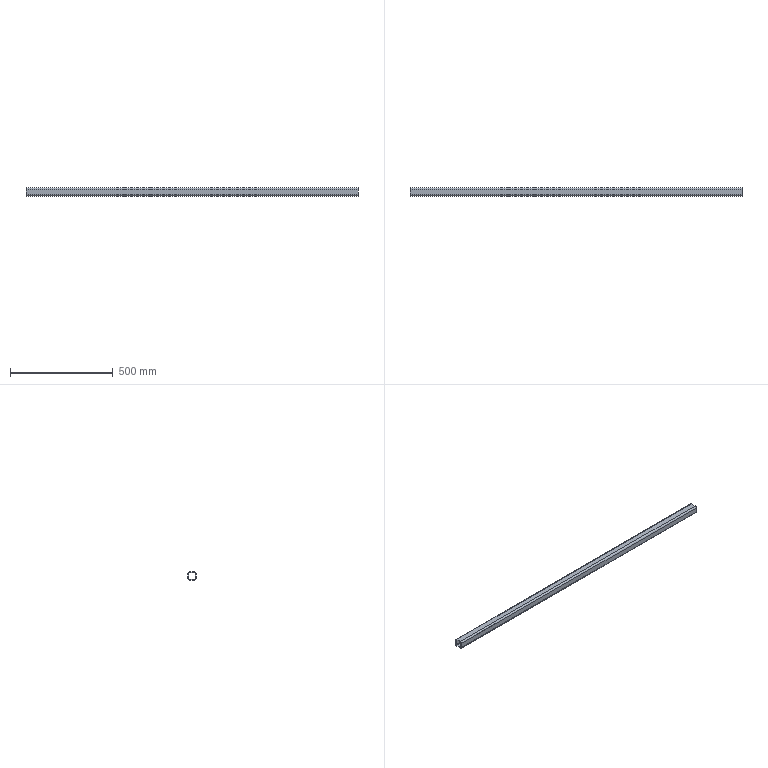Part | STEP file | Microwave Drying Flat Conveyor-CN2500x400-105-102_Default<Machining blank> | 1 solid | 18 faces | box 1612 x 40 x 40 mm | volume 862092 mm3 | plane 10 | cylinder 8 | commonest cylinder face diameters 8 x4 16 x4
STEP:
#1=CARTESIAN_POINT('',(0.,-20.,12.));
#2=VERTEX_POINT('',#1);
#3=CARTESIAN_POINT('',(0.,-12.,20.));
#4=VERTEX_POINT('',#3);
#5=CARTESIAN_POINT('',(0.,-12.,12.));
#6=DIRECTION('',(-1.,0.,0.));
#7=DIRECTION('',(0.,-1.,0.));
#8=AXIS2_PLACEMENT_3D('',#5,#6,#7);
#9=CIRCLE('',#8,8.);
#10=EDGE_CURVE('',#2,#4,#9,.T.);
#11=ORIENTED_EDGE('',*,*,#10,.T.);
#12=CARTESIAN_POINT('',(-1612.,-12.,20.));
#13=VERTEX_POINT('',#12);
#14=CARTESIAN_POINT('',(-1612.,-12.,20.));
#15=DIRECTION('',(1.,0.,0.));
#16=VECTOR('',#15,1000.);
#17=LINE('',#14,#16);
#18=EDGE_CURVE('',#13,#4,#17,.T.);
#19=ORIENTED_EDGE('',*,*,#18,.F.);
#20=CARTESIAN_POINT('',(-1612.,-20.,12.));
#21=VERTEX_POINT('',#20);
#22=CARTESIAN_POINT('',(-1612.,-12.,12.));
#23=DIRECTION('',(-1.,0.,0.));
#24=DIRECTION('',(0.,-1.,0.));
#25=AXIS2_PLACEMENT_3D('',#22,#23,#24);
#26=CIRCLE('',#25,8.);
#27=EDGE_CURVE('',#21,#13,#26,.T.);
#28=ORIENTED_EDGE('',*,*,#27,.F.);
#29=CARTESIAN_POINT('',(-1612.,-20.,12.));
#30=DIRECTION('',(1.,0.,0.));
#31=VECTOR('',#30,1000.);
#32=LINE('',#29,#31);
#33=EDGE_CURVE('',#21,#2,#32,.T.);
#34=ORIENTED_EDGE('',*,*,#33,.T.);
#35=EDGE_LOOP('',(#11,#19,#28,#34));
#36=FACE_OUTER_BOUND('',#35,.T.);
#37=CARTESIAN_POINT('',(-1612.,-12.,12.));
#38=DIRECTION('',(1.,0.,0.));
#39=DIRECTION('',(0.,1.,0.));
#40=AXIS2_PLACEMENT_3D('',#37,#38,#39);
#41=CYLINDRICAL_SURFACE('',#40,8.);
#42=ADVANCED_FACE('',(#36),#41,.T.);
#43=CARTESIAN_POINT('',(0.,12.,20.));
#44=VERTEX_POINT('',#43);
#45=CARTESIAN_POINT('',(0.,-12.,20.));
#46=DIRECTION('',(0.,1.,0.));
#47=VECTOR('',#46,1000.);
#48=LINE('',#45,#47);
#49=EDGE_CURVE('',#4,#44,#48,.T.);
#50=ORIENTED_EDGE('',*,*,#49,.T.);
#51=CARTESIAN_POINT('',(-1612.,12.,20.));
#52=VERTEX_POINT('',#51);
#53=CARTESIAN_POINT('',(-1612.,12.,20.));
#54=DIRECTION('',(1.,0.,0.));
#55=VECTOR('',#54,1000.);
#56=LINE('',#53,#55);
#57=EDGE_CURVE('',#52,#44,#56,.T.);
#58=ORIENTED_EDGE('',*,*,#57,.F.);
#59=CARTESIAN_POINT('',(-1612.,-12.,20.));
#60=DIRECTION('',(0.,1.,0.));
#61=VECTOR('',#60,1000.);
#62=LINE('',#59,#61);
#63=EDGE_CURVE('',#13,#52,#62,.T.);
#64=ORIENTED_EDGE('',*,*,#63,.F.);
#65=ORIENTED_EDGE('',*,*,#18,.T.);
#66=EDGE_LOOP('',(#50,#58,#64,#65));
#67=FACE_OUTER_BOUND('',#66,.T.);
#68=CARTESIAN_POINT('',(-1612.,-12.,20.));
#69=DIRECTION('',(0.,0.,-1.));
#70=DIRECTION('',(-1.,0.,0.));
#71=AXIS2_PLACEMENT_3D('',#68,#69,#70);
#72=PLANE('',#71);
#73=ADVANCED_FACE('',(#67),#72,.F.);
#74=CARTESIAN_POINT('',(0.,20.,12.));
#75=VERTEX_POINT('',#74);
#76=CARTESIAN_POINT('',(0.,12.,12.));
#77=DIRECTION('',(-1.,0.,0.));
#78=DIRECTION('',(0.,-1.,0.));
#79=AXIS2_PLACEMENT_3D('',#76,#77,#78);
#80=CIRCLE('',#79,8.);
#81=EDGE_CURVE('',#44,#75,#80,.T.);
#82=ORIENTED_EDGE('',*,*,#81,.T.);
#83=CARTESIAN_POINT('',(-1612.,20.,12.));
#84=VERTEX_POINT('',#83);
#85=CARTESIAN_POINT('',(-1612.,20.,12.));
#86=DIRECTION('',(1.,0.,0.));
#87=VECTOR('',#86,1000.);
#88=LINE('',#85,#87);
#89=EDGE_CURVE('',#84,#75,#88,.T.);
#90=ORIENTED_EDGE('',*,*,#89,.F.);
#91=CARTESIAN_POINT('',(-1612.,12.,12.));
#92=DIRECTION('',(-1.,0.,0.));
#93=DIRECTION('',(0.,-1.,0.));
#94=AXIS2_PLACEMENT_3D('',#91,#92,#93);
#95=CIRCLE('',#94,8.);
#96=EDGE_CURVE('',#52,#84,#95,.T.);
#97=ORIENTED_EDGE('',*,*,#96,.F.);
#98=ORIENTED_EDGE('',*,*,#57,.T.);
#99=EDGE_LOOP('',(#82,#90,#97,#98));
#100=FACE_OUTER_BOUND('',#99,.T.);
#101=CARTESIAN_POINT('',(-1612.,12.,12.));
#102=DIRECTION('',(1.,0.,0.));
#103=DIRECTION('',(0.,1.,0.));
#104=AXIS2_PLACEMENT_3D('',#101,#102,#103);
#105=CYLINDRICAL_SURFACE('',#104,8.);
#106=ADVANCED_FACE('',(#100),#105,.T.);
#107=CARTESIAN_POINT('',(0.,20.,-12.));
#108=VERTEX_POINT('',#107);
#109=CARTESIAN_POINT('',(0.,20.,-12.));
#110=DIRECTION('',(0.,0.,-1.));
#111=VECTOR('',#110,1000.);
#112=LINE('',#109,#111);
#113=EDGE_CURVE('',#75,#108,#112,.T.);
#114=ORIENTED_EDGE('',*,*,#113,.T.);
#115=CARTESIAN_POINT('',(-1612.,20.,-12.));
#116=VERTEX_POINT('',#115);
#117=CARTESIAN_POINT('',(-1612.,20.,-12.));
#118=DIRECTION('',(1.,0.,0.));
#119=VECTOR('',#118,1000.);
#120=LINE('',#117,#119);
#121=EDGE_CURVE('',#116,#108,#120,.T.);
#122=ORIENTED_EDGE('',*,*,#121,.F.);
#123=CARTESIAN_POINT('',(-1612.,20.,-12.));
#124=DIRECTION('',(0.,0.,-1.));
#125=VECTOR('',#124,1000.);
#126=LINE('',#123,#125);
#127=EDGE_CURVE('',#84,#116,#126,.T.);
#128=ORIENTED_EDGE('',*,*,#127,.F.);
#129=ORIENTED_EDGE('',*,*,#89,.T.);
#130=EDGE_LOOP('',(#114,#122,#128,#129));
#131=FACE_OUTER_BOUND('',#130,.T.);
#132=CARTESIAN_POINT('',(-1612.,20.,-12.));
#133=DIRECTION('',(0.,-1.,0.));
#134=DIRECTION('',(1.,0.,0.));
#135=AXIS2_PLACEMENT_3D('',#132,#133,#134);
#136=PLANE('',#135);
#137=ADVANCED_FACE('',(#131),#136,.F.);
#138=CARTESIAN_POINT('',(0.,12.,-20.));
#139=VERTEX_POINT('',#138);
#140=CARTESIAN_POINT('',(0.,12.,-12.));
#141=DIRECTION('',(-1.,0.,0.));
#142=DIRECTION('',(0.,-1.,0.));
#143=AXIS2_PLACEMENT_3D('',#140,#141,#142);
#144=CIRCLE('',#143,8.);
#145=EDGE_CURVE('',#108,#139,#144,.T.);
#146=ORIENTED_EDGE('',*,*,#145,.T.);
#147=CARTESIAN_POINT('',(-1612.,12.,-20.));
#148=VERTEX_POINT('',#147);
#149=CARTESIAN_POINT('',(-1612.,12.,-20.));
#150=DIRECTION('',(1.,0.,0.));
#151=VECTOR('',#150,1000.);
#152=LINE('',#149,#151);
#153=EDGE_CURVE('',#148,#139,#152,.T.);
#154=ORIENTED_EDGE('',*,*,#153,.F.);
#155=CARTESIAN_POINT('',(-1612.,12.,-12.));
#156=DIRECTION('',(-1.,0.,0.));
#157=DIRECTION('',(0.,-1.,0.));
#158=AXIS2_PLACEMENT_3D('',#155,#156,#157);
#159=CIRCLE('',#158,8.);
#160=EDGE_CURVE('',#116,#148,#159,.T.);
#161=ORIENTED_EDGE('',*,*,#160,.F.);
#162=ORIENTED_EDGE('',*,*,#121,.T.);
#163=EDGE_LOOP('',(#146,#154,#161,#162));
#164=FACE_OUTER_BOUND('',#163,.T.);
#165=CARTESIAN_POINT('',(-1612.,12.,-12.));
#166=DIRECTION('',(1.,0.,0.));
#167=DIRECTION('',(0.,1.,0.));
#168=AXIS2_PLACEMENT_3D('',#165,#166,#167);
#169=CYLINDRICAL_SURFACE('',#168,8.);
#170=ADVANCED_FACE('',(#164),#169,.T.);
#171=CARTESIAN_POINT('',(0.,-12.,-20.));
#172=VERTEX_POINT('',#171);
#173=CARTESIAN_POINT('',(0.,12.,-20.));
#174=DIRECTION('',(0.,-1.,0.));
#175=VECTOR('',#174,1000.);
#176=LINE('',#173,#175);
#177=EDGE_CURVE('',#139,#172,#176,.T.);
#178=ORIENTED_EDGE('',*,*,#177,.T.);
#179=CARTESIAN_POINT('',(-1612.,-12.,-20.));
#180=VERTEX_POINT('',#179);
#181=CARTESIAN_POINT('',(-1612.,-12.,-20.));
#182=DIRECTION('',(1.,0.,0.));
#183=VECTOR('',#182,1000.);
#184=LINE('',#181,#183);
#185=EDGE_CURVE('',#180,#172,#184,.T.);
#186=ORIENTED_EDGE('',*,*,#185,.F.);
#187=CARTESIAN_POINT('',(-1612.,12.,-20.));
#188=DIRECTION('',(0.,-1.,0.));
#189=VECTOR('',#188,1000.);
#190=LINE('',#187,#189);
#191=EDGE_CURVE('',#148,#180,#190,.T.);
#192=ORIENTED_EDGE('',*,*,#191,.F.);
#193=ORIENTED_EDGE('',*,*,#153,.T.);
#194=EDGE_LOOP('',(#178,#186,#192,#193));
#195=FACE_OUTER_BOUND('',#194,.T.);
#196=CARTESIAN_POINT('',(-1612.,12.,-20.));
#197=DIRECTION('',(0.,0.,1.));
#198=DIRECTION('',(1.,0.,0.));
#199=AXIS2_PLACEMENT_3D('',#196,#197,#198);
#200=PLANE('',#199);
#201=ADVANCED_FACE('',(#195),#200,.F.);
#202=CARTESIAN_POINT('',(0.,-20.,-12.));
#203=VERTEX_POINT('',#202);
#204=CARTESIAN_POINT('',(0.,-12.,-12.));
#205=DIRECTION('',(-1.,0.,0.));
#206=DIRECTION('',(0.,-1.,0.));
#207=AXIS2_PLACEMENT_3D('',#204,#205,#206);
#208=CIRCLE('',#207,8.);
#209=EDGE_CURVE('',#172,#203,#208,.T.);
#210=ORIENTED_EDGE('',*,*,#209,.T.);
#211=CARTESIAN_POINT('',(-1612.,-20.,-12.));
#212=VERTEX_POINT('',#211);
#213=CARTESIAN_POINT('',(-1612.,-20.,-12.));
#214=DIRECTION('',(1.,0.,0.));
#215=VECTOR('',#214,1000.);
#216=LINE('',#213,#215);
#217=EDGE_CURVE('',#212,#203,#216,.T.);
#218=ORIENTED_EDGE('',*,*,#217,.F.);
#219=CARTESIAN_POINT('',(-1612.,-12.,-12.));
#220=DIRECTION('',(-1.,0.,0.));
#221=DIRECTION('',(0.,-1.,0.));
#222=AXIS2_PLACEMENT_3D('',#219,#220,#221);
#223=CIRCLE('',#222,8.);
#224=EDGE_CURVE('',#180,#212,#223,.T.);
#225=ORIENTED_EDGE('',*,*,#224,.F.);
#226=ORIENTED_EDGE('',*,*,#185,.T.);
#227=EDGE_LOOP('',(#210,#218,#225,#226));
#228=FACE_OUTER_BOUND('',#227,.T.);
#229=CARTESIAN_POINT('',(-1612.,-12.,-12.));
#230=DIRECTION('',(1.,0.,0.));
#231=DIRECTION('',(0.,1.,0.));
#232=AXIS2_PLACEMENT_3D('',#229,#230,#231);
#233=CYLINDRICAL_SURFACE('',#232,8.);
#234=ADVANCED_FACE('',(#228),#233,.T.);
#235=CARTESIAN_POINT('',(0.,12.,16.));
#236=VERTEX_POINT('',#235);
#237=CARTESIAN_POINT('',(0.,16.,12.));
#238=VERTEX_POINT('',#237);
#239=CARTESIAN_POINT('',(0.,12.,12.));
#240=DIRECTION('',(-1.,0.,0.));
#241=DIRECTION('',(0.,-1.,0.));
#242=AXIS2_PLACEMENT_3D('',#239,#240,#241);
#243=CIRCLE('',#242,4.);
#244=EDGE_CURVE('',#236,#238,#243,.T.);
#245=ORIENTED_EDGE('',*,*,#244,.F.);
#246=CARTESIAN_POINT('',(-1612.,12.,16.));
#247=VERTEX_POINT('',#246);
#248=CARTESIAN_POINT('',(-1612.,12.,16.));
#249=DIRECTION('',(1.,0.,0.));
#250=VECTOR('',#249,1000.);
#251=LINE('',#248,#250);
#252=EDGE_CURVE('',#247,#236,#251,.T.);
#253=ORIENTED_EDGE('',*,*,#252,.F.);
#254=CARTESIAN_POINT('',(-1612.,16.,12.));
#255=VERTEX_POINT('',#254);
#256=CARTESIAN_POINT('',(-1612.,12.,12.));
#257=DIRECTION('',(-1.,0.,0.));
#258=DIRECTION('',(0.,-1.,0.));
#259=AXIS2_PLACEMENT_3D('',#256,#257,#258);
#260=CIRCLE('',#259,4.);
#261=EDGE_CURVE('',#247,#255,#260,.T.);
#262=ORIENTED_EDGE('',*,*,#261,.T.);
#263=CARTESIAN_POINT('',(-1612.,16.,12.));
#264=DIRECTION('',(1.,0.,0.));
#265=VECTOR('',#264,1000.);
#266=LINE('',#263,#265);
#267=EDGE_CURVE('',#255,#238,#266,.T.);
#268=ORIENTED_EDGE('',*,*,#267,.T.);
#269=EDGE_LOOP('',(#245,#253,#262,#268));
#270=FACE_OUTER_BOUND('',#269,.T.);
#271=CARTESIAN_POINT('',(-1612.,12.,12.));
#272=DIRECTION('',(1.,0.,0.));
#273=DIRECTION('',(0.,1.,0.));
#274=AXIS2_PLACEMENT_3D('',#271,#272,#273);
#275=CYLINDRICAL_SURFACE('',#274,4.);
#276=ADVANCED_FACE('',(#270),#275,.F.);
#277=CARTESIAN_POINT('',(0.,-12.,16.));
#278=VERTEX_POINT('',#277);
#279=CARTESIAN_POINT('',(0.,-12.,16.));
#280=DIRECTION('',(0.,1.,0.));
#281=VECTOR('',#280,1000.);
#282=LINE('',#279,#281);
#283=EDGE_CURVE('',#278,#236,#282,.T.);
#284=ORIENTED_EDGE('',*,*,#283,.F.);
#285=CARTESIAN_POINT('',(-1612.,-12.,16.));
#286=VERTEX_POINT('',#285);
#287=CARTESIAN_POINT('',(-1612.,-12.,16.));
#288=DIRECTION('',(1.,0.,0.));
#289=VECTOR('',#288,1000.);
#290=LINE('',#287,#289);
#291=EDGE_CURVE('',#286,#278,#290,.T.);
#292=ORIENTED_EDGE('',*,*,#291,.F.);
#293=CARTESIAN_POINT('',(-1612.,-12.,16.));
#294=DIRECTION('',(0.,1.,0.));
#295=VECTOR('',#294,1000.);
#296=LINE('',#293,#295);
#297=EDGE_CURVE('',#286,#247,#296,.T.);
#298=ORIENTED_EDGE('',*,*,#297,.T.);
#299=ORIENTED_EDGE('',*,*,#252,.T.);
#300=EDGE_LOOP('',(#284,#292,#298,#299));
#301=FACE_OUTER_BOUND('',#300,.T.);
#302=CARTESIAN_POINT('',(-1612.,-12.,16.));
#303=DIRECTION('',(0.,0.,-1.));
#304=DIRECTION('',(-1.,0.,0.));
#305=AXIS2_PLACEMENT_3D('',#302,#303,#304);
#306=PLANE('',#305);
#307=ADVANCED_FACE('',(#301),#306,.T.);
#308=CARTESIAN_POINT('',(0.,-16.,12.));
#309=VERTEX_POINT('',#308);
#310=CARTESIAN_POINT('',(0.,-12.,12.));
#311=DIRECTION('',(-1.,0.,0.));
#312=DIRECTION('',(0.,-1.,0.));
#313=AXIS2_PLACEMENT_3D('',#310,#311,#312);
#314=CIRCLE('',#313,4.);
#315=EDGE_CURVE('',#309,#278,#314,.T.);
#316=ORIENTED_EDGE('',*,*,#315,.F.);
#317=CARTESIAN_POINT('',(-1612.,-16.,12.));
#318=VERTEX_POINT('',#317);
#319=CARTESIAN_POINT('',(-1612.,-16.,12.));
#320=DIRECTION('',(1.,0.,0.));
#321=VECTOR('',#320,1000.);
#322=LINE('',#319,#321);
#323=EDGE_CURVE('',#318,#309,#322,.T.);
#324=ORIENTED_EDGE('',*,*,#323,.F.);
#325=CARTESIAN_POINT('',(-1612.,-12.,12.));
#326=DIRECTION('',(-1.,0.,0.));
#327=DIRECTION('',(0.,-1.,0.));
#328=AXIS2_PLACEMENT_3D('',#325,#326,#327);
#329=CIRCLE('',#328,4.);
#330=EDGE_CURVE('',#318,#286,#329,.T.);
#331=ORIENTED_EDGE('',*,*,#330,.T.);
#332=ORIENTED_EDGE('',*,*,#291,.T.);
#333=EDGE_LOOP('',(#316,#324,#331,#332));
#334=FACE_OUTER_BOUND('',#333,.T.);
#335=CARTESIAN_POINT('',(-1612.,-12.,12.));
#336=DIRECTION('',(1.,0.,0.));
#337=DIRECTION('',(0.,1.,0.));
#338=AXIS2_PLACEMENT_3D('',#335,#336,#337);
#339=CYLINDRICAL_SURFACE('',#338,4.);
#340=ADVANCED_FACE('',(#334),#339,.F.);
#341=CARTESIAN_POINT('',(0.,-16.,-12.));
#342=VERTEX_POINT('',#341);
#343=CARTESIAN_POINT('',(0.,-16.,12.));
#344=DIRECTION('',(0.,0.,1.));
#345=VECTOR('',#344,1000.);
#346=LINE('',#343,#345);
#347=EDGE_CURVE('',#342,#309,#346,.T.);
#348=ORIENTED_EDGE('',*,*,#347,.F.);
#349=CARTESIAN_POINT('',(-1612.,-16.,-12.));
#350=VERTEX_POINT('',#349);
#351=CARTESIAN_POINT('',(-1612.,-16.,-12.));
#352=DIRECTION('',(1.,0.,0.));
#353=VECTOR('',#352,1000.);
#354=LINE('',#351,#353);
#355=EDGE_CURVE('',#350,#342,#354,.T.);
#356=ORIENTED_EDGE('',*,*,#355,.F.);
#357=CARTESIAN_POINT('',(-1612.,-16.,12.));
#358=DIRECTION('',(0.,0.,1.));
#359=VECTOR('',#358,1000.);
#360=LINE('',#357,#359);
#361=EDGE_CURVE('',#350,#318,#360,.T.);
#362=ORIENTED_EDGE('',*,*,#361,.T.);
#363=ORIENTED_EDGE('',*,*,#323,.T.);
#364=EDGE_LOOP('',(#348,#356,#362,#363));
#365=FACE_OUTER_BOUND('',#364,.T.);
#366=CARTESIAN_POINT('',(-1612.,-16.,12.));
#367=DIRECTION('',(0.,1.,0.));
#368=DIRECTION('',(-1.,0.,0.));
#369=AXIS2_PLACEMENT_3D('',#366,#367,#368);
#370=PLANE('',#369);
#371=ADVANCED_FACE('',(#365),#370,.T.);
#372=CARTESIAN_POINT('',(0.,-12.,-16.));
#373=VERTEX_POINT('',#372);
#374=CARTESIAN_POINT('',(0.,-12.,-12.));
#375=DIRECTION('',(-1.,0.,0.));
#376=DIRECTION('',(0.,-1.,0.));
#377=AXIS2_PLACEMENT_3D('',#374,#375,#376);
#378=CIRCLE('',#377,4.);
#379=EDGE_CURVE('',#373,#342,#378,.T.);
#380=ORIENTED_EDGE('',*,*,#379,.F.);
#381=CARTESIAN_POINT('',(-1612.,-12.,-16.));
#382=VERTEX_POINT('',#381);
#383=CARTESIAN_POINT('',(-1612.,-12.,-16.));
#384=DIRECTION('',(1.,0.,0.));
#385=VECTOR('',#384,1000.);
#386=LINE('',#383,#385);
#387=EDGE_CURVE('',#382,#373,#386,.T.);
#388=ORIENTED_EDGE('',*,*,#387,.F.);
#389=CARTESIAN_POINT('',(-1612.,-12.,-12.));
#390=DIRECTION('',(-1.,0.,0.));
#391=DIRECTION('',(0.,-1.,0.));
#392=AXIS2_PLACEMENT_3D('',#389,#390,#391);
#393=CIRCLE('',#392,4.);
#394=EDGE_CURVE('',#382,#350,#393,.T.);
#395=ORIENTED_EDGE('',*,*,#394,.T.);
#396=ORIENTED_EDGE('',*,*,#355,.T.);
#397=EDGE_LOOP('',(#380,#388,#395,#396));
#398=FACE_OUTER_BOUND('',#397,.T.);
#399=CARTESIAN_POINT('',(-1612.,-12.,-12.));
#400=DIRECTION('',(1.,0.,0.));
#401=DIRECTION('',(0.,1.,0.));
#402=AXIS2_PLACEMENT_3D('',#399,#400,#401);
#403=CYLINDRICAL_SURFACE('',#402,4.);
#404=ADVANCED_FACE('',(#398),#403,.F.);
#405=CARTESIAN_POINT('',(0.,12.,-16.));
#406=VERTEX_POINT('',#405);
#407=CARTESIAN_POINT('',(0.,12.,-16.));
#408=DIRECTION('',(0.,-1.,0.));
#409=VECTOR('',#408,1000.);
#410=LINE('',#407,#409);
#411=EDGE_CURVE('',#406,#373,#410,.T.);
#412=ORIENTED_EDGE('',*,*,#411,.F.);
#413=CARTESIAN_POINT('',(-1612.,12.,-16.));
#414=VERTEX_POINT('',#413);
#415=CARTESIAN_POINT('',(-1612.,12.,-16.));
#416=DIRECTION('',(1.,0.,0.));
#417=VECTOR('',#416,1000.);
#418=LINE('',#415,#417);
#419=EDGE_CURVE('',#414,#406,#418,.T.);
#420=ORIENTED_EDGE('',*,*,#419,.F.);
#421=CARTESIAN_POINT('',(-1612.,12.,-16.));
#422=DIRECTION('',(0.,-1.,0.));
#423=VECTOR('',#422,1000.);
#424=LINE('',#421,#423);
#425=EDGE_CURVE('',#414,#382,#424,.T.);
#426=ORIENTED_EDGE('',*,*,#425,.T.);
#427=ORIENTED_EDGE('',*,*,#387,.T.);
#428=EDGE_LOOP('',(#412,#420,#426,#427));
#429=FACE_OUTER_BOUND('',#428,.T.);
#430=CARTESIAN_POINT('',(-1612.,12.,-16.));
#431=DIRECTION('',(0.,0.,1.));
#432=DIRECTION('',(1.,0.,0.));
#433=AXIS2_PLACEMENT_3D('',#430,#431,#432);
#434=PLANE('',#433);
#435=ADVANCED_FACE('',(#429),#434,.T.);
#436=CARTESIAN_POINT('',(0.,16.,-12.));
#437=VERTEX_POINT('',#436);
#438=CARTESIAN_POINT('',(0.,12.,-12.));
#439=DIRECTION('',(-1.,0.,0.));
#440=DIRECTION('',(0.,-1.,0.));
#441=AXIS2_PLACEMENT_3D('',#438,#439,#440);
#442=CIRCLE('',#441,4.);
#443=EDGE_CURVE('',#437,#406,#442,.T.);
#444=ORIENTED_EDGE('',*,*,#443,.F.);
#445=CARTESIAN_POINT('',(-1612.,16.,-12.));
#446=VERTEX_POINT('',#445);
#447=CARTESIAN_POINT('',(-1612.,16.,-12.));
#448=DIRECTION('',(1.,0.,0.));
#449=VECTOR('',#448,1000.);
#450=LINE('',#447,#449);
#451=EDGE_CURVE('',#446,#437,#450,.T.);
#452=ORIENTED_EDGE('',*,*,#451,.F.);
#453=CARTESIAN_POINT('',(-1612.,12.,-12.));
#454=DIRECTION('',(-1.,0.,0.));
#455=DIRECTION('',(0.,-1.,0.));
#456=AXIS2_PLACEMENT_3D('',#453,#454,#455);
#457=CIRCLE('',#456,4.);
#458=EDGE_CURVE('',#446,#414,#457,.T.);
#459=ORIENTED_EDGE('',*,*,#458,.T.);
#460=ORIENTED_EDGE('',*,*,#419,.T.);
#461=EDGE_LOOP('',(#444,#452,#459,#460));
#462=FACE_OUTER_BOUND('',#461,.T.);
#463=CARTESIAN_POINT('',(-1612.,12.,-12.));
#464=DIRECTION('',(1.,0.,0.));
#465=DIRECTION('',(0.,1.,0.));
#466=AXIS2_PLACEMENT_3D('',#463,#464,#465);
#467=CYLINDRICAL_SURFACE('',#466,4.);
#468=ADVANCED_FACE('',(#462),#467,.F.);
#469=CARTESIAN_POINT('',(0.,16.,-12.));
#470=DIRECTION('',(0.,0.,-1.));
#471=VECTOR('',#470,1000.);
#472=LINE('',#469,#471);
#473=EDGE_CURVE('',#238,#437,#472,.T.);
#474=ORIENTED_EDGE('',*,*,#473,.F.);
#475=ORIENTED_EDGE('',*,*,#267,.F.);
#476=CARTESIAN_POINT('',(-1612.,16.,-12.));
#477=DIRECTION('',(0.,0.,-1.));
#478=VECTOR('',#477,1000.);
#479=LINE('',#476,#478);
#480=EDGE_CURVE('',#255,#446,#479,.T.);
#481=ORIENTED_EDGE('',*,*,#480,.T.);
#482=ORIENTED_EDGE('',*,*,#451,.T.);
#483=EDGE_LOOP('',(#474,#475,#481,#482));
#484=FACE_OUTER_BOUND('',#483,.T.);
#485=CARTESIAN_POINT('',(-1612.,16.,-12.));
#486=DIRECTION('',(0.,-1.,0.));
#487=DIRECTION('',(1.,0.,0.));
#488=AXIS2_PLACEMENT_3D('',#485,#486,#487);
#489=PLANE('',#488);
#490=ADVANCED_FACE('',(#484),#489,.T.);
#491=CARTESIAN_POINT('',(0.,-20.,12.));
#492=DIRECTION('',(0.,0.,1.));
#493=VECTOR('',#492,1000.);
#494=LINE('',#491,#493);
#495=EDGE_CURVE('',#203,#2,#494,.T.);
#496=ORIENTED_EDGE('',*,*,#495,.T.);
#497=ORIENTED_EDGE('',*,*,#33,.F.);
#498=CARTESIAN_POINT('',(-1612.,-20.,12.));
#499=DIRECTION('',(0.,0.,1.));
#500=VECTOR('',#499,1000.);
#501=LINE('',#498,#500);
#502=EDGE_CURVE('',#212,#21,#501,.T.);
#503=ORIENTED_EDGE('',*,*,#502,.F.);
#504=ORIENTED_EDGE('',*,*,#217,.T.);
#505=EDGE_LOOP('',(#496,#497,#503,#504));
#506=FACE_OUTER_BOUND('',#505,.T.);
#507=CARTESIAN_POINT('',(-1612.,-20.,12.));
#508=DIRECTION('',(0.,1.,0.));
#509=DIRECTION('',(-1.,0.,0.));
#510=AXIS2_PLACEMENT_3D('',#507,#508,#509);
#511=PLANE('',#510);
#512=ADVANCED_FACE('',(#506),#511,.F.);
#513=ORIENTED_EDGE('',*,*,#261,.F.);
#514=ORIENTED_EDGE('',*,*,#297,.F.);
#515=ORIENTED_EDGE('',*,*,#330,.F.);
#516=ORIENTED_EDGE('',*,*,#361,.F.);
#517=ORIENTED_EDGE('',*,*,#394,.F.);
#518=ORIENTED_EDGE('',*,*,#425,.F.);
#519=ORIENTED_EDGE('',*,*,#458,.F.);
#520=ORIENTED_EDGE('',*,*,#480,.F.);
#521=EDGE_LOOP('',(#513,#514,#515,#516,#517,#518,#519,#520));
#522=FACE_BOUND('',#521,.T.);
#523=ORIENTED_EDGE('',*,*,#27,.T.);
#524=ORIENTED_EDGE('',*,*,#63,.T.);
#525=ORIENTED_EDGE('',*,*,#96,.T.);
#526=ORIENTED_EDGE('',*,*,#127,.T.);
#527=ORIENTED_EDGE('',*,*,#160,.T.);
#528=ORIENTED_EDGE('',*,*,#191,.T.);
#529=ORIENTED_EDGE('',*,*,#224,.T.);
#530=ORIENTED_EDGE('',*,*,#502,.T.);
#531=EDGE_LOOP('',(#523,#524,#525,#526,#527,#528,#529,#530));
#532=FACE_OUTER_BOUND('',#531,.T.);
#533=CARTESIAN_POINT('',(-1612.,-12.,12.));
#534=DIRECTION('',(-1.,0.,0.));
#535=DIRECTION('',(0.,-1.,0.));
#536=AXIS2_PLACEMENT_3D('',#533,#534,#535);
#537=PLANE('',#536);
#538=ADVANCED_FACE('',(#522,#532),#537,.T.);
#539=ORIENTED_EDGE('',*,*,#244,.T.);
#540=ORIENTED_EDGE('',*,*,#473,.T.);
#541=ORIENTED_EDGE('',*,*,#443,.T.);
#542=ORIENTED_EDGE('',*,*,#411,.T.);
#543=ORIENTED_EDGE('',*,*,#379,.T.);
#544=ORIENTED_EDGE('',*,*,#347,.T.);
#545=ORIENTED_EDGE('',*,*,#315,.T.);
#546=ORIENTED_EDGE('',*,*,#283,.T.);
#547=EDGE_LOOP('',(#539,#540,#541,#542,#543,#544,#545,#546));
#548=FACE_BOUND('',#547,.T.);
#549=ORIENTED_EDGE('',*,*,#10,.F.);
#550=ORIENTED_EDGE('',*,*,#495,.F.);
#551=ORIENTED_EDGE('',*,*,#209,.F.);
#552=ORIENTED_EDGE('',*,*,#177,.F.);
#553=ORIENTED_EDGE('',*,*,#145,.F.);
#554=ORIENTED_EDGE('',*,*,#113,.F.);
#555=ORIENTED_EDGE('',*,*,#81,.F.);
#556=ORIENTED_EDGE('',*,*,#49,.F.);
#557=EDGE_LOOP('',(#549,#550,#551,#552,#553,#554,#555,#556));
#558=FACE_OUTER_BOUND('',#557,.T.);
#559=CARTESIAN_POINT('',(0.,-12.,12.));
#560=DIRECTION('',(-1.,0.,0.));
#561=DIRECTION('',(0.,-1.,0.));
#562=AXIS2_PLACEMENT_3D('',#559,#560,#561);
#563=PLANE('',#562);
#564=ADVANCED_FACE('',(#548,#558),#563,.F.);
#565=CLOSED_SHELL('',(#42,#73,#106,#137,#170,#201,#234,#276,#307,#340,#371,#404,#435,#468,#490,#512,#538,#564));
#566=MANIFOLD_SOLID_BREP('',#565);
#567=CARTESIAN_POINT('',(0.,0.,0.));
#568=DIRECTION('',(0.,0.,1.));
#569=DIRECTION('',(1.,0.,0.));
#570=AXIS2_PLACEMENT_3D('',#567,#568,#569);
#571=(LENGTH_UNIT()NAMED_UNIT(*)SI_UNIT(.MILLI.,.METRE.));
#572=UNCERTAINTY_MEASURE_WITH_UNIT(LENGTH_MEASURE(0.00001),#571,'','');
#573=(NAMED_UNIT(*)PLANE_ANGLE_UNIT()SI_UNIT($,.RADIAN.));
#574=(NAMED_UNIT(*)SI_UNIT($,.STERADIAN.)SOLID_ANGLE_UNIT());
#575=(GEOMETRIC_REPRESENTATION_CONTEXT(3)GLOBAL_UNCERTAINTY_ASSIGNED_CONTEXT((#572))GLOBAL_UNIT_ASSIGNED_CONTEXT((#571,#573,#574))REPRESENTATION_CONTEXT('',''));
#576=ADVANCED_BREP_SHAPE_REPRESENTATION('',(#566,#570),#575);